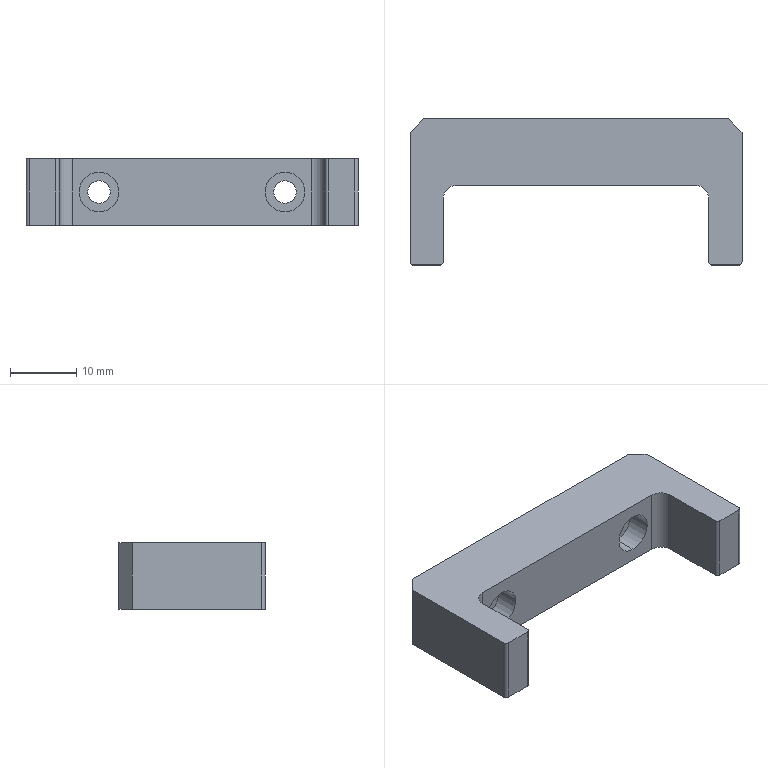Part | SolidWorks | features Fillet 2, Chamfer 1, Extrusion 1, HoleWzd 1 | 1 solid | 28 faces | box 50 x 22 x 10 mm | volume 5859 mm3 | cylinder 14 | plane 14 | commonest cylinder face diameters 1 x4 3.4 x4 6 x4 4 x2
STEP:
#1=CARTESIAN_POINT('',(11.,-6.5,8.));
#2=VERTEX_POINT('',#1);
#3=CARTESIAN_POINT('',(11.,-6.5,2.));
#4=VERTEX_POINT('',#3);
#5=CARTESIAN_POINT('',(11.,-6.5,5.));
#6=DIRECTION('',(0.,-1.,0.));
#7=DIRECTION('',(0.,0.,-1.));
#8=AXIS2_PLACEMENT_3D('',#5,#6,#7);
#9=CIRCLE('',#8,3.);
#10=EDGE_CURVE('',#2,#4,#9,.T.);
#11=ORIENTED_EDGE('',*,*,#10,.F.);
#12=CARTESIAN_POINT('',(11.,-10.,8.));
#13=VERTEX_POINT('',#12);
#14=CARTESIAN_POINT('',(11.,-10.,8.));
#15=DIRECTION('',(0.,-1.,0.));
#16=VECTOR('',#15,1000.);
#17=LINE('',#14,#16);
#18=EDGE_CURVE('',#2,#13,#17,.T.);
#19=ORIENTED_EDGE('',*,*,#18,.T.);
#20=CARTESIAN_POINT('',(11.,-10.,2.));
#21=VERTEX_POINT('',#20);
#22=CARTESIAN_POINT('',(11.,-10.,5.));
#23=DIRECTION('',(0.,-1.,0.));
#24=DIRECTION('',(0.,0.,-1.));
#25=AXIS2_PLACEMENT_3D('',#22,#23,#24);
#26=CIRCLE('',#25,3.);
#27=EDGE_CURVE('',#13,#21,#26,.T.);
#28=ORIENTED_EDGE('',*,*,#27,.T.);
#29=CARTESIAN_POINT('',(11.,-10.,2.));
#30=DIRECTION('',(0.,-1.,0.));
#31=VECTOR('',#30,1000.);
#32=LINE('',#29,#31);
#33=EDGE_CURVE('',#4,#21,#32,.T.);
#34=ORIENTED_EDGE('',*,*,#33,.F.);
#35=EDGE_LOOP('',(#11,#19,#28,#34));
#36=FACE_OUTER_BOUND('',#35,.T.);
#37=CARTESIAN_POINT('',(11.,-10.,5.));
#38=DIRECTION('',(0.,-1.,0.));
#39=DIRECTION('',(0.,0.,-1.));
#40=AXIS2_PLACEMENT_3D('',#37,#38,#39);
#41=CYLINDRICAL_SURFACE('',#40,3.);
#42=ADVANCED_FACE('',(#36),#41,.F.);
#43=CARTESIAN_POINT('',(11.,0.,6.7));
#44=VERTEX_POINT('',#43);
#45=CARTESIAN_POINT('',(11.,0.,3.3));
#46=VERTEX_POINT('',#45);
#47=CARTESIAN_POINT('',(11.,0.,5.));
#48=DIRECTION('',(0.,-1.,0.));
#49=DIRECTION('',(0.,0.,-1.));
#50=AXIS2_PLACEMENT_3D('',#47,#48,#49);
#51=CIRCLE('',#50,1.7);
#52=EDGE_CURVE('',#44,#46,#51,.T.);
#53=ORIENTED_EDGE('',*,*,#52,.F.);
#54=CARTESIAN_POINT('',(11.,-6.5,6.7));
#55=VERTEX_POINT('',#54);
#56=CARTESIAN_POINT('',(11.,-10.,6.7));
#57=DIRECTION('',(0.,-1.,0.));
#58=VECTOR('',#57,1000.);
#59=LINE('',#56,#58);
#60=EDGE_CURVE('',#44,#55,#59,.T.);
#61=ORIENTED_EDGE('',*,*,#60,.T.);
#62=CARTESIAN_POINT('',(11.,-6.5,3.3));
#63=VERTEX_POINT('',#62);
#64=CARTESIAN_POINT('',(11.,-6.5,5.));
#65=DIRECTION('',(0.,-1.,0.));
#66=DIRECTION('',(0.,0.,-1.));
#67=AXIS2_PLACEMENT_3D('',#64,#65,#66);
#68=CIRCLE('',#67,1.7);
#69=EDGE_CURVE('',#55,#63,#68,.T.);
#70=ORIENTED_EDGE('',*,*,#69,.T.);
#71=CARTESIAN_POINT('',(11.,-10.,3.3));
#72=DIRECTION('',(0.,-1.,0.));
#73=VECTOR('',#72,1000.);
#74=LINE('',#71,#73);
#75=EDGE_CURVE('',#46,#63,#74,.T.);
#76=ORIENTED_EDGE('',*,*,#75,.F.);
#77=EDGE_LOOP('',(#53,#61,#70,#76));
#78=FACE_OUTER_BOUND('',#77,.T.);
#79=CARTESIAN_POINT('',(11.,-10.,5.));
#80=DIRECTION('',(0.,-1.,0.));
#81=DIRECTION('',(0.,0.,-1.));
#82=AXIS2_PLACEMENT_3D('',#79,#80,#81);
#83=CYLINDRICAL_SURFACE('',#82,1.7);
#84=ADVANCED_FACE('',(#78),#83,.F.);
#85=CARTESIAN_POINT('',(39.,-6.5,8.));
#86=VERTEX_POINT('',#85);
#87=CARTESIAN_POINT('',(39.,-6.5,2.));
#88=VERTEX_POINT('',#87);
#89=CARTESIAN_POINT('',(39.,-6.5,5.));
#90=DIRECTION('',(0.,-1.,0.));
#91=DIRECTION('',(0.,0.,-1.));
#92=AXIS2_PLACEMENT_3D('',#89,#90,#91);
#93=CIRCLE('',#92,3.);
#94=EDGE_CURVE('',#86,#88,#93,.T.);
#95=ORIENTED_EDGE('',*,*,#94,.F.);
#96=CARTESIAN_POINT('',(39.,-10.,8.));
#97=VERTEX_POINT('',#96);
#98=CARTESIAN_POINT('',(39.,-10.,8.));
#99=DIRECTION('',(0.,-1.,0.));
#100=VECTOR('',#99,1000.);
#101=LINE('',#98,#100);
#102=EDGE_CURVE('',#86,#97,#101,.T.);
#103=ORIENTED_EDGE('',*,*,#102,.T.);
#104=CARTESIAN_POINT('',(39.,-10.,2.));
#105=VERTEX_POINT('',#104);
#106=CARTESIAN_POINT('',(39.,-10.,5.));
#107=DIRECTION('',(0.,-1.,0.));
#108=DIRECTION('',(0.,0.,-1.));
#109=AXIS2_PLACEMENT_3D('',#106,#107,#108);
#110=CIRCLE('',#109,3.);
#111=EDGE_CURVE('',#97,#105,#110,.T.);
#112=ORIENTED_EDGE('',*,*,#111,.T.);
#113=CARTESIAN_POINT('',(39.,-10.,2.));
#114=DIRECTION('',(0.,-1.,0.));
#115=VECTOR('',#114,1000.);
#116=LINE('',#113,#115);
#117=EDGE_CURVE('',#88,#105,#116,.T.);
#118=ORIENTED_EDGE('',*,*,#117,.F.);
#119=EDGE_LOOP('',(#95,#103,#112,#118));
#120=FACE_OUTER_BOUND('',#119,.T.);
#121=CARTESIAN_POINT('',(39.,-10.,5.));
#122=DIRECTION('',(0.,-1.,0.));
#123=DIRECTION('',(0.,0.,-1.));
#124=AXIS2_PLACEMENT_3D('',#121,#122,#123);
#125=CYLINDRICAL_SURFACE('',#124,3.);
#126=ADVANCED_FACE('',(#120),#125,.F.);
#127=CARTESIAN_POINT('',(39.,0.,6.7));
#128=VERTEX_POINT('',#127);
#129=CARTESIAN_POINT('',(39.,0.,3.3));
#130=VERTEX_POINT('',#129);
#131=CARTESIAN_POINT('',(39.,0.,5.));
#132=DIRECTION('',(0.,-1.,0.));
#133=DIRECTION('',(0.,0.,-1.));
#134=AXIS2_PLACEMENT_3D('',#131,#132,#133);
#135=CIRCLE('',#134,1.7);
#136=EDGE_CURVE('',#128,#130,#135,.T.);
#137=ORIENTED_EDGE('',*,*,#136,.F.);
#138=CARTESIAN_POINT('',(39.,-6.5,6.7));
#139=VERTEX_POINT('',#138);
#140=CARTESIAN_POINT('',(39.,-10.,6.7));
#141=DIRECTION('',(0.,-1.,0.));
#142=VECTOR('',#141,1000.);
#143=LINE('',#140,#142);
#144=EDGE_CURVE('',#128,#139,#143,.T.);
#145=ORIENTED_EDGE('',*,*,#144,.T.);
#146=CARTESIAN_POINT('',(39.,-6.5,3.3));
#147=VERTEX_POINT('',#146);
#148=CARTESIAN_POINT('',(39.,-6.5,5.));
#149=DIRECTION('',(0.,-1.,0.));
#150=DIRECTION('',(0.,0.,-1.));
#151=AXIS2_PLACEMENT_3D('',#148,#149,#150);
#152=CIRCLE('',#151,1.7);
#153=EDGE_CURVE('',#139,#147,#152,.T.);
#154=ORIENTED_EDGE('',*,*,#153,.T.);
#155=CARTESIAN_POINT('',(39.,-10.,3.3));
#156=DIRECTION('',(0.,-1.,0.));
#157=VECTOR('',#156,1000.);
#158=LINE('',#155,#157);
#159=EDGE_CURVE('',#130,#147,#158,.T.);
#160=ORIENTED_EDGE('',*,*,#159,.F.);
#161=EDGE_LOOP('',(#137,#145,#154,#160));
#162=FACE_OUTER_BOUND('',#161,.T.);
#163=CARTESIAN_POINT('',(39.,-10.,5.));
#164=DIRECTION('',(0.,-1.,0.));
#165=DIRECTION('',(0.,0.,-1.));
#166=AXIS2_PLACEMENT_3D('',#163,#164,#165);
#167=CYLINDRICAL_SURFACE('',#166,1.7);
#168=ADVANCED_FACE('',(#162),#167,.F.);
#169=CARTESIAN_POINT('',(0.,-2.,10.));
#170=VERTEX_POINT('',#169);
#171=CARTESIAN_POINT('',(0.,-21.5,10.));
#172=VERTEX_POINT('',#171);
#173=CARTESIAN_POINT('',(0.,0.,10.));
#174=DIRECTION('',(0.,-1.,0.));
#175=VECTOR('',#174,1000.);
#176=LINE('',#173,#175);
#177=EDGE_CURVE('',#170,#172,#176,.T.);
#178=ORIENTED_EDGE('',*,*,#177,.F.);
#179=CARTESIAN_POINT('',(0.,-2.,0.));
#180=VERTEX_POINT('',#179);
#181=CARTESIAN_POINT('',(0.,-2.,10.));
#182=DIRECTION('',(0.,0.,-1.));
#183=VECTOR('',#182,1000.);
#184=LINE('',#181,#183);
#185=EDGE_CURVE('',#170,#180,#184,.T.);
#186=ORIENTED_EDGE('',*,*,#185,.T.);
#187=CARTESIAN_POINT('',(0.,-21.5,0.));
#188=VERTEX_POINT('',#187);
#189=CARTESIAN_POINT('',(0.,0.,0.));
#190=DIRECTION('',(0.,-1.,0.));
#191=VECTOR('',#190,1000.);
#192=LINE('',#189,#191);
#193=EDGE_CURVE('',#180,#188,#192,.T.);
#194=ORIENTED_EDGE('',*,*,#193,.T.);
#195=CARTESIAN_POINT('',(0.,-21.5,10.));
#196=DIRECTION('',(0.,0.,1.));
#197=VECTOR('',#196,1000.);
#198=LINE('',#195,#197);
#199=EDGE_CURVE('',#188,#172,#198,.T.);
#200=ORIENTED_EDGE('',*,*,#199,.T.);
#201=EDGE_LOOP('',(#178,#186,#194,#200));
#202=FACE_OUTER_BOUND('',#201,.T.);
#203=CARTESIAN_POINT('',(0.,0.,10.));
#204=DIRECTION('',(1.,0.,0.));
#205=DIRECTION('',(0.,1.,0.));
#206=AXIS2_PLACEMENT_3D('',#203,#204,#205);
#207=PLANE('',#206);
#208=ADVANCED_FACE('',(#202),#207,.F.);
#209=CARTESIAN_POINT('',(0.5,-22.,0.));
#210=VERTEX_POINT('',#209);
#211=CARTESIAN_POINT('',(4.5,-22.,0.));
#212=VERTEX_POINT('',#211);
#213=CARTESIAN_POINT('',(0.,-22.,0.));
#214=DIRECTION('',(1.,0.,0.));
#215=VECTOR('',#214,1000.);
#216=LINE('',#213,#215);
#217=EDGE_CURVE('',#210,#212,#216,.T.);
#218=ORIENTED_EDGE('',*,*,#217,.T.);
#219=CARTESIAN_POINT('',(4.5,-22.,10.));
#220=VERTEX_POINT('',#219);
#221=CARTESIAN_POINT('',(4.5,-22.,10.));
#222=DIRECTION('',(0.,0.,1.));
#223=VECTOR('',#222,1000.);
#224=LINE('',#221,#223);
#225=EDGE_CURVE('',#212,#220,#224,.T.);
#226=ORIENTED_EDGE('',*,*,#225,.T.);
#227=CARTESIAN_POINT('',(0.5,-22.,10.));
#228=VERTEX_POINT('',#227);
#229=CARTESIAN_POINT('',(0.,-22.,10.));
#230=DIRECTION('',(1.,0.,0.));
#231=VECTOR('',#230,1000.);
#232=LINE('',#229,#231);
#233=EDGE_CURVE('',#228,#220,#232,.T.);
#234=ORIENTED_EDGE('',*,*,#233,.F.);
#235=CARTESIAN_POINT('',(0.5,-22.,10.));
#236=DIRECTION('',(0.,0.,-1.));
#237=VECTOR('',#236,1000.);
#238=LINE('',#235,#237);
#239=EDGE_CURVE('',#228,#210,#238,.T.);
#240=ORIENTED_EDGE('',*,*,#239,.T.);
#241=EDGE_LOOP('',(#218,#226,#234,#240));
#242=FACE_OUTER_BOUND('',#241,.T.);
#243=CARTESIAN_POINT('',(0.,-22.,10.));
#244=DIRECTION('',(0.,1.,0.));
#245=DIRECTION('',(0.,0.,1.));
#246=AXIS2_PLACEMENT_3D('',#243,#244,#245);
#247=PLANE('',#246);
#248=ADVANCED_FACE('',(#242),#247,.F.);
#249=CARTESIAN_POINT('',(5.,-21.5,10.));
#250=VERTEX_POINT('',#249);
#251=CARTESIAN_POINT('',(5.,-12.,10.));
#252=VERTEX_POINT('',#251);
#253=CARTESIAN_POINT('',(5.,-22.,10.));
#254=DIRECTION('',(0.,1.,0.));
#255=VECTOR('',#254,1000.);
#256=LINE('',#253,#255);
#257=EDGE_CURVE('',#250,#252,#256,.T.);
#258=ORIENTED_EDGE('',*,*,#257,.F.);
#259=CARTESIAN_POINT('',(5.,-21.5,0.));
#260=VERTEX_POINT('',#259);
#261=CARTESIAN_POINT('',(5.,-21.5,10.));
#262=DIRECTION('',(0.,0.,-1.));
#263=VECTOR('',#262,1000.);
#264=LINE('',#261,#263);
#265=EDGE_CURVE('',#250,#260,#264,.T.);
#266=ORIENTED_EDGE('',*,*,#265,.T.);
#267=CARTESIAN_POINT('',(5.,-12.,0.));
#268=VERTEX_POINT('',#267);
#269=CARTESIAN_POINT('',(5.,-22.,0.));
#270=DIRECTION('',(0.,1.,0.));
#271=VECTOR('',#270,1000.);
#272=LINE('',#269,#271);
#273=EDGE_CURVE('',#260,#268,#272,.T.);
#274=ORIENTED_EDGE('',*,*,#273,.T.);
#275=CARTESIAN_POINT('',(5.,-12.,10.));
#276=DIRECTION('',(0.,0.,1.));
#277=VECTOR('',#276,1000.);
#278=LINE('',#275,#277);
#279=EDGE_CURVE('',#268,#252,#278,.T.);
#280=ORIENTED_EDGE('',*,*,#279,.T.);
#281=EDGE_LOOP('',(#258,#266,#274,#280));
#282=FACE_OUTER_BOUND('',#281,.T.);
#283=CARTESIAN_POINT('',(5.,-22.,10.));
#284=DIRECTION('',(-1.,0.,0.));
#285=DIRECTION('',(0.,0.,1.));
#286=AXIS2_PLACEMENT_3D('',#283,#284,#285);
#287=PLANE('',#286);
#288=ADVANCED_FACE('',(#282),#287,.F.);
#289=CARTESIAN_POINT('',(11.,-10.,5.));
#290=DIRECTION('',(0.,-1.,0.));
#291=DIRECTION('',(0.,0.,-1.));
#292=AXIS2_PLACEMENT_3D('',#289,#290,#291);
#293=CIRCLE('',#292,3.);
#294=EDGE_CURVE('',#21,#13,#293,.T.);
#295=ORIENTED_EDGE('',*,*,#294,.F.);
#296=ORIENTED_EDGE('',*,*,#27,.F.);
#297=EDGE_LOOP('',(#295,#296));
#298=FACE_BOUND('',#297,.T.);
#299=CARTESIAN_POINT('',(39.,-10.,5.));
#300=DIRECTION('',(0.,-1.,0.));
#301=DIRECTION('',(0.,0.,-1.));
#302=AXIS2_PLACEMENT_3D('',#299,#300,#301);
#303=CIRCLE('',#302,3.);
#304=EDGE_CURVE('',#105,#97,#303,.T.);
#305=ORIENTED_EDGE('',*,*,#304,.F.);
#306=ORIENTED_EDGE('',*,*,#111,.F.);
#307=EDGE_LOOP('',(#305,#306));
#308=FACE_BOUND('',#307,.T.);
#309=CARTESIAN_POINT('',(7.,-10.,0.));
#310=VERTEX_POINT('',#309);
#311=CARTESIAN_POINT('',(43.,-10.,0.));
#312=VERTEX_POINT('',#311);
#313=CARTESIAN_POINT('',(5.,-10.,0.));
#314=DIRECTION('',(1.,0.,0.));
#315=VECTOR('',#314,1000.);
#316=LINE('',#313,#315);
#317=EDGE_CURVE('',#310,#312,#316,.T.);
#318=ORIENTED_EDGE('',*,*,#317,.T.);
#319=CARTESIAN_POINT('',(43.,-10.,10.));
#320=VERTEX_POINT('',#319);
#321=CARTESIAN_POINT('',(43.,-10.,10.));
#322=DIRECTION('',(0.,0.,1.));
#323=VECTOR('',#322,1000.);
#324=LINE('',#321,#323);
#325=EDGE_CURVE('',#312,#320,#324,.T.);
#326=ORIENTED_EDGE('',*,*,#325,.T.);
#327=CARTESIAN_POINT('',(7.,-10.,10.));
#328=VERTEX_POINT('',#327);
#329=CARTESIAN_POINT('',(5.,-10.,10.));
#330=DIRECTION('',(1.,0.,0.));
#331=VECTOR('',#330,1000.);
#332=LINE('',#329,#331);
#333=EDGE_CURVE('',#328,#320,#332,.T.);
#334=ORIENTED_EDGE('',*,*,#333,.F.);
#335=CARTESIAN_POINT('',(7.,-10.,0.));
#336=DIRECTION('',(0.,0.,-1.));
#337=VECTOR('',#336,1000.);
#338=LINE('',#335,#337);
#339=EDGE_CURVE('',#328,#310,#338,.T.);
#340=ORIENTED_EDGE('',*,*,#339,.T.);
#341=EDGE_LOOP('',(#318,#326,#334,#340));
#342=FACE_OUTER_BOUND('',#341,.T.);
#343=CARTESIAN_POINT('',(5.,-10.,10.));
#344=DIRECTION('',(0.,1.,0.));
#345=DIRECTION('',(0.,0.,1.));
#346=AXIS2_PLACEMENT_3D('',#343,#344,#345);
#347=PLANE('',#346);
#348=ADVANCED_FACE('',(#298,#308,#342),#347,.F.);
#349=CARTESIAN_POINT('',(45.,-12.,0.));
#350=VERTEX_POINT('',#349);
#351=CARTESIAN_POINT('',(45.,-21.5,0.));
#352=VERTEX_POINT('',#351);
#353=CARTESIAN_POINT('',(45.,-22.,0.));
#354=DIRECTION('',(0.,-1.,0.));
#355=VECTOR('',#354,1000.);
#356=LINE('',#353,#355);
#357=EDGE_CURVE('',#350,#352,#356,.T.);
#358=ORIENTED_EDGE('',*,*,#357,.T.);
#359=CARTESIAN_POINT('',(45.,-21.5,10.));
#360=VERTEX_POINT('',#359);
#361=CARTESIAN_POINT('',(45.,-21.5,10.));
#362=DIRECTION('',(0.,0.,1.));
#363=VECTOR('',#362,1000.);
#364=LINE('',#361,#363);
#365=EDGE_CURVE('',#352,#360,#364,.T.);
#366=ORIENTED_EDGE('',*,*,#365,.T.);
#367=CARTESIAN_POINT('',(45.,-12.,10.));
#368=VERTEX_POINT('',#367);
#369=CARTESIAN_POINT('',(45.,-22.,10.));
#370=DIRECTION('',(0.,-1.,0.));
#371=VECTOR('',#370,1000.);
#372=LINE('',#369,#371);
#373=EDGE_CURVE('',#368,#360,#372,.T.);
#374=ORIENTED_EDGE('',*,*,#373,.F.);
#375=CARTESIAN_POINT('',(45.,-12.,0.));
#376=DIRECTION('',(0.,0.,-1.));
#377=VECTOR('',#376,1000.);
#378=LINE('',#375,#377);
#379=EDGE_CURVE('',#368,#350,#378,.T.);
#380=ORIENTED_EDGE('',*,*,#379,.T.);
#381=EDGE_LOOP('',(#358,#366,#374,#380));
#382=FACE_OUTER_BOUND('',#381,.T.);
#383=CARTESIAN_POINT('',(45.,-22.,10.));
#384=DIRECTION('',(1.,0.,0.));
#385=DIRECTION('',(0.,0.,-1.));
#386=AXIS2_PLACEMENT_3D('',#383,#384,#385);
#387=PLANE('',#386);
#388=ADVANCED_FACE('',(#382),#387,.F.);
#389=CARTESIAN_POINT('',(45.5,-22.,0.));
#390=VERTEX_POINT('',#389);
#391=CARTESIAN_POINT('',(49.5,-22.,0.));
#392=VERTEX_POINT('',#391);
#393=CARTESIAN_POINT('',(45.,-22.,0.));
#394=DIRECTION('',(1.,0.,0.));
#395=VECTOR('',#394,1000.);
#396=LINE('',#393,#395);
#397=EDGE_CURVE('',#390,#392,#396,.T.);
#398=ORIENTED_EDGE('',*,*,#397,.T.);
#399=CARTESIAN_POINT('',(49.5,-22.,10.));
#400=VERTEX_POINT('',#399);
#401=CARTESIAN_POINT('',(49.5,-22.,10.));
#402=DIRECTION('',(0.,0.,1.));
#403=VECTOR('',#402,1000.);
#404=LINE('',#401,#403);
#405=EDGE_CURVE('',#392,#400,#404,.T.);
#406=ORIENTED_EDGE('',*,*,#405,.T.);
#407=CARTESIAN_POINT('',(45.5,-22.,10.));
#408=VERTEX_POINT('',#407);
#409=CARTESIAN_POINT('',(45.,-22.,10.));
#410=DIRECTION('',(1.,0.,0.));
#411=VECTOR('',#410,1000.);
#412=LINE('',#409,#411);
#413=EDGE_CURVE('',#408,#400,#412,.T.);
#414=ORIENTED_EDGE('',*,*,#413,.F.);
#415=CARTESIAN_POINT('',(45.5,-22.,10.));
#416=DIRECTION('',(0.,0.,-1.));
#417=VECTOR('',#416,1000.);
#418=LINE('',#415,#417);
#419=EDGE_CURVE('',#408,#390,#418,.T.);
#420=ORIENTED_EDGE('',*,*,#419,.T.);
#421=EDGE_LOOP('',(#398,#406,#414,#420));
#422=FACE_OUTER_BOUND('',#421,.T.);
#423=CARTESIAN_POINT('',(45.,-22.,10.));
#424=DIRECTION('',(0.,1.,0.));
#425=DIRECTION('',(0.,0.,1.));
#426=AXIS2_PLACEMENT_3D('',#423,#424,#425);
#427=PLANE('',#426);
#428=ADVANCED_FACE('',(#422),#427,.F.);
#429=CARTESIAN_POINT('',(50.,-21.5,0.));
#430=VERTEX_POINT('',#429);
#431=CARTESIAN_POINT('',(50.,-2.,0.));
#432=VERTEX_POINT('',#431);
#433=CARTESIAN_POINT('',(50.,0.,0.));
#434=DIRECTION('',(0.,1.,0.));
#435=VECTOR('',#434,1000.);
#436=LINE('',#433,#435);
#437=EDGE_CURVE('',#430,#432,#436,.T.);
#438=ORIENTED_EDGE('',*,*,#437,.T.);
#439=CARTESIAN_POINT('',(50.,-2.,10.));
#440=VERTEX_POINT('',#439);
#441=CARTESIAN_POINT('',(50.,-2.,10.));
#442=DIRECTION('',(0.,0.,1.));
#443=VECTOR('',#442,1000.);
#444=LINE('',#441,#443);
#445=EDGE_CURVE('',#432,#440,#444,.T.);
#446=ORIENTED_EDGE('',*,*,#445,.T.);
#447=CARTESIAN_POINT('',(50.,-21.5,10.));
#448=VERTEX_POINT('',#447);
#449=CARTESIAN_POINT('',(50.,0.,10.));
#450=DIRECTION('',(0.,1.,0.));
#451=VECTOR('',#450,1000.);
#452=LINE('',#449,#451);
#453=EDGE_CURVE('',#448,#440,#452,.T.);
#454=ORIENTED_EDGE('',*,*,#453,.F.);
#455=CARTESIAN_POINT('',(50.,-21.5,10.));
#456=DIRECTION('',(0.,0.,-1.));
#457=VECTOR('',#456,1000.);
#458=LINE('',#455,#457);
#459=EDGE_CURVE('',#448,#430,#458,.T.);
#460=ORIENTED_EDGE('',*,*,#459,.T.);
#461=EDGE_LOOP('',(#438,#446,#454,#460));
#462=FACE_OUTER_BOUND('',#461,.T.);
#463=CARTESIAN_POINT('',(50.,0.,10.));
#464=DIRECTION('',(-1.,0.,0.));
#465=DIRECTION('',(0.,0.,1.));
#466=AXIS2_PLACEMENT_3D('',#463,#464,#465);
#467=PLANE('',#466);
#468=ADVANCED_FACE('',(#462),#467,.F.);
#469=CARTESIAN_POINT('',(11.,0.,5.));
#470=DIRECTION('',(0.,-1.,0.));
#471=DIRECTION('',(0.,0.,-1.));
#472=AXIS2_PLACEMENT_3D('',#469,#470,#471);
#473=CIRCLE('',#472,1.7);
#474=EDGE_CURVE('',#46,#44,#473,.T.);
#475=ORIENTED_EDGE('',*,*,#474,.T.);
#476=ORIENTED_EDGE('',*,*,#52,.T.);
#477=EDGE_LOOP('',(#475,#476));
#478=FACE_BOUND('',#477,.T.);
#479=CARTESIAN_POINT('',(39.,0.,5.));
#480=DIRECTION('',(0.,-1.,0.));
#481=DIRECTION('',(0.,0.,-1.));
#482=AXIS2_PLACEMENT_3D('',#479,#480,#481);
#483=CIRCLE('',#482,1.7);
#484=EDGE_CURVE('',#130,#128,#483,.T.);
#485=ORIENTED_EDGE('',*,*,#484,.T.);
#486=ORIENTED_EDGE('',*,*,#136,.T.);
#487=EDGE_LOOP('',(#485,#486));
#488=FACE_BOUND('',#487,.T.);
#489=CARTESIAN_POINT('',(48.,0.,10.));
#490=VERTEX_POINT('',#489);
#491=CARTESIAN_POINT('',(2.,0.,10.));
#492=VERTEX_POINT('',#491);
#493=CARTESIAN_POINT('',(0.,0.,10.));
#494=DIRECTION('',(-1.,0.,0.));
#495=VECTOR('',#494,1000.);
#496=LINE('',#493,#495);
#497=EDGE_CURVE('',#490,#492,#496,.T.);
#498=ORIENTED_EDGE('',*,*,#497,.F.);
#499=CARTESIAN_POINT('',(48.,0.,0.));
#500=VERTEX_POINT('',#499);
#501=CARTESIAN_POINT('',(48.,0.,10.));
#502=DIRECTION('',(0.,0.,-1.));
#503=VECTOR('',#502,1000.);
#504=LINE('',#501,#503);
#505=EDGE_CURVE('',#490,#500,#504,.T.);
#506=ORIENTED_EDGE('',*,*,#505,.T.);
#507=CARTESIAN_POINT('',(2.,0.,0.));
#508=VERTEX_POINT('',#507);
#509=CARTESIAN_POINT('',(0.,0.,0.));
#510=DIRECTION('',(-1.,0.,0.));
#511=VECTOR('',#510,1000.);
#512=LINE('',#509,#511);
#513=EDGE_CURVE('',#500,#508,#512,.T.);
#514=ORIENTED_EDGE('',*,*,#513,.T.);
#515=CARTESIAN_POINT('',(2.,0.,10.));
#516=DIRECTION('',(0.,0.,1.));
#517=VECTOR('',#516,1000.);
#518=LINE('',#515,#517);
#519=EDGE_CURVE('',#508,#492,#518,.T.);
#520=ORIENTED_EDGE('',*,*,#519,.T.);
#521=EDGE_LOOP('',(#498,#506,#514,#520));
#522=FACE_OUTER_BOUND('',#521,.T.);
#523=CARTESIAN_POINT('',(0.,0.,10.));
#524=DIRECTION('',(0.,-1.,0.));
#525=DIRECTION('',(0.,0.,-1.));
#526=AXIS2_PLACEMENT_3D('',#523,#524,#525);
#527=PLANE('',#526);
#528=ADVANCED_FACE('',(#478,#488,#522),#527,.F.);
#529=ORIENTED_EDGE('',*,*,#453,.T.);
#530=CARTESIAN_POINT('',(35.,13.,10.));
#531=DIRECTION('',(-0.7071,0.7071,0.));
#532=VECTOR('',#531,1000.);
#533=LINE('',#530,#532);
#534=EDGE_CURVE('',#440,#490,#533,.T.);
#535=ORIENTED_EDGE('',*,*,#534,.T.);
#536=ORIENTED_EDGE('',*,*,#497,.T.);
#537=CARTESIAN_POINT('',(-10.,-12.,10.));
#538=DIRECTION('',(-0.7071,-0.7071,0.));
#539=VECTOR('',#538,1000.);
#540=LINE('',#537,#539);
#541=EDGE_CURVE('',#492,#170,#540,.T.);
#542=ORIENTED_EDGE('',*,*,#541,.T.);
#543=ORIENTED_EDGE('',*,*,#177,.T.);
#544=CARTESIAN_POINT('',(0.5,-21.5,10.));
#545=DIRECTION('',(0.,0.,1.));
#546=DIRECTION('',(1.,0.,0.));
#547=AXIS2_PLACEMENT_3D('',#544,#545,#546);
#548=CIRCLE('',#547,0.5);
#549=EDGE_CURVE('',#172,#228,#548,.T.);
#550=ORIENTED_EDGE('',*,*,#549,.T.);
#551=ORIENTED_EDGE('',*,*,#233,.T.);
#552=CARTESIAN_POINT('',(4.5,-21.5,10.));
#553=DIRECTION('',(0.,0.,1.));
#554=DIRECTION('',(1.,0.,0.));
#555=AXIS2_PLACEMENT_3D('',#552,#553,#554);
#556=CIRCLE('',#555,0.5);
#557=EDGE_CURVE('',#220,#250,#556,.T.);
#558=ORIENTED_EDGE('',*,*,#557,.T.);
#559=ORIENTED_EDGE('',*,*,#257,.T.);
#560=CARTESIAN_POINT('',(7.,-12.,10.));
#561=DIRECTION('',(0.,0.,-1.));
#562=DIRECTION('',(1.,0.,0.));
#563=AXIS2_PLACEMENT_3D('',#560,#561,#562);
#564=CIRCLE('',#563,2.);
#565=EDGE_CURVE('',#252,#328,#564,.T.);
#566=ORIENTED_EDGE('',*,*,#565,.T.);
#567=ORIENTED_EDGE('',*,*,#333,.T.);
#568=CARTESIAN_POINT('',(43.,-12.,10.));
#569=DIRECTION('',(0.,0.,-1.));
#570=DIRECTION('',(1.,0.,0.));
#571=AXIS2_PLACEMENT_3D('',#568,#569,#570);
#572=CIRCLE('',#571,2.);
#573=EDGE_CURVE('',#320,#368,#572,.T.);
#574=ORIENTED_EDGE('',*,*,#573,.T.);
#575=ORIENTED_EDGE('',*,*,#373,.T.);
#576=CARTESIAN_POINT('',(45.5,-21.5,10.));
#577=DIRECTION('',(0.,0.,1.));
#578=DIRECTION('',(1.,0.,0.));
#579=AXIS2_PLACEMENT_3D('',#576,#577,#578);
#580=CIRCLE('',#579,0.5);
#581=EDGE_CURVE('',#360,#408,#580,.T.);
#582=ORIENTED_EDGE('',*,*,#581,.T.);
#583=ORIENTED_EDGE('',*,*,#413,.T.);
#584=CARTESIAN_POINT('',(49.5,-21.5,10.));
#585=DIRECTION('',(0.,0.,1.));
#586=DIRECTION('',(1.,0.,0.));
#587=AXIS2_PLACEMENT_3D('',#584,#585,#586);
#588=CIRCLE('',#587,0.5);
#589=EDGE_CURVE('',#400,#448,#588,.T.);
#590=ORIENTED_EDGE('',*,*,#589,.T.);
#591=EDGE_LOOP('',(#529,#535,#536,#542,#543,#550,#551,#558,#559,#566,#567,#574,#575,#582,#583,#590));
#592=FACE_OUTER_BOUND('',#591,.T.);
#593=CARTESIAN_POINT('',(0.,-22.,10.));
#594=DIRECTION('',(0.,0.,1.));
#595=DIRECTION('',(1.,0.,0.));
#596=AXIS2_PLACEMENT_3D('',#593,#594,#595);
#597=PLANE('',#596);
#598=ADVANCED_FACE('',(#592),#597,.T.);
#599=ORIENTED_EDGE('',*,*,#513,.F.);
#600=CARTESIAN_POINT('',(48.,0.,0.));
#601=DIRECTION('',(0.7071,-0.7071,0.));
#602=VECTOR('',#601,1000.);
#603=LINE('',#600,#602);
#604=EDGE_CURVE('',#500,#432,#603,.T.);
#605=ORIENTED_EDGE('',*,*,#604,.T.);
#606=ORIENTED_EDGE('',*,*,#437,.F.);
#607=CARTESIAN_POINT('',(49.5,-21.5,0.));
#608=DIRECTION('',(0.,0.,-1.));
#609=DIRECTION('',(1.,0.,0.));
#610=AXIS2_PLACEMENT_3D('',#607,#608,#609);
#611=CIRCLE('',#610,0.5);
#612=EDGE_CURVE('',#430,#392,#611,.T.);
#613=ORIENTED_EDGE('',*,*,#612,.T.);
#614=ORIENTED_EDGE('',*,*,#397,.F.);
#615=CARTESIAN_POINT('',(45.5,-21.5,0.));
#616=DIRECTION('',(0.,0.,-1.));
#617=DIRECTION('',(1.,0.,0.));
#618=AXIS2_PLACEMENT_3D('',#615,#616,#617);
#619=CIRCLE('',#618,0.5);
#620=EDGE_CURVE('',#390,#352,#619,.T.);
#621=ORIENTED_EDGE('',*,*,#620,.T.);
#622=ORIENTED_EDGE('',*,*,#357,.F.);
#623=CARTESIAN_POINT('',(43.,-12.,0.));
#624=DIRECTION('',(0.,0.,1.));
#625=DIRECTION('',(1.,0.,0.));
#626=AXIS2_PLACEMENT_3D('',#623,#624,#625);
#627=CIRCLE('',#626,2.);
#628=EDGE_CURVE('',#350,#312,#627,.T.);
#629=ORIENTED_EDGE('',*,*,#628,.T.);
#630=ORIENTED_EDGE('',*,*,#317,.F.);
#631=CARTESIAN_POINT('',(7.,-12.,0.));
#632=DIRECTION('',(0.,0.,1.));
#633=DIRECTION('',(1.,0.,0.));
#634=AXIS2_PLACEMENT_3D('',#631,#632,#633);
#635=CIRCLE('',#634,2.);
#636=EDGE_CURVE('',#310,#268,#635,.T.);
#637=ORIENTED_EDGE('',*,*,#636,.T.);
#638=ORIENTED_EDGE('',*,*,#273,.F.);
#639=CARTESIAN_POINT('',(4.5,-21.5,0.));
#640=DIRECTION('',(0.,0.,-1.));
#641=DIRECTION('',(1.,0.,0.));
#642=AXIS2_PLACEMENT_3D('',#639,#640,#641);
#643=CIRCLE('',#642,0.5);
#644=EDGE_CURVE('',#260,#212,#643,.T.);
#645=ORIENTED_EDGE('',*,*,#644,.T.);
#646=ORIENTED_EDGE('',*,*,#217,.F.);
#647=CARTESIAN_POINT('',(0.5,-21.5,0.));
#648=DIRECTION('',(0.,0.,-1.));
#649=DIRECTION('',(1.,0.,0.));
#650=AXIS2_PLACEMENT_3D('',#647,#648,#649);
#651=CIRCLE('',#650,0.5);
#652=EDGE_CURVE('',#210,#188,#651,.T.);
#653=ORIENTED_EDGE('',*,*,#652,.T.);
#654=ORIENTED_EDGE('',*,*,#193,.F.);
#655=CARTESIAN_POINT('',(0.,-2.,0.));
#656=DIRECTION('',(0.7071,0.7071,0.));
#657=VECTOR('',#656,1000.);
#658=LINE('',#655,#657);
#659=EDGE_CURVE('',#180,#508,#658,.T.);
#660=ORIENTED_EDGE('',*,*,#659,.T.);
#661=EDGE_LOOP('',(#599,#605,#606,#613,#614,#621,#622,#629,#630,#637,#638,#645,#646,#653,#654,#660));
#662=FACE_OUTER_BOUND('',#661,.T.);
#663=CARTESIAN_POINT('',(0.,-22.,0.));
#664=DIRECTION('',(0.,0.,1.));
#665=DIRECTION('',(1.,0.,0.));
#666=AXIS2_PLACEMENT_3D('',#663,#664,#665);
#667=PLANE('',#666);
#668=ADVANCED_FACE('',(#662),#667,.F.);
#669=ORIENTED_EDGE('',*,*,#144,.F.);
#670=ORIENTED_EDGE('',*,*,#484,.F.);
#671=ORIENTED_EDGE('',*,*,#159,.T.);
#672=CARTESIAN_POINT('',(39.,-6.5,5.));
#673=DIRECTION('',(0.,-1.,0.));
#674=DIRECTION('',(0.,0.,-1.));
#675=AXIS2_PLACEMENT_3D('',#672,#673,#674);
#676=CIRCLE('',#675,1.7);
#677=EDGE_CURVE('',#147,#139,#676,.T.);
#678=ORIENTED_EDGE('',*,*,#677,.T.);
#679=EDGE_LOOP('',(#669,#670,#671,#678));
#680=FACE_OUTER_BOUND('',#679,.T.);
#681=CARTESIAN_POINT('',(39.,-10.,5.));
#682=DIRECTION('',(0.,-1.,0.));
#683=DIRECTION('',(0.,0.,-1.));
#684=AXIS2_PLACEMENT_3D('',#681,#682,#683);
#685=CYLINDRICAL_SURFACE('',#684,1.7);
#686=ADVANCED_FACE('',(#680),#685,.F.);
#687=ORIENTED_EDGE('',*,*,#677,.F.);
#688=ORIENTED_EDGE('',*,*,#153,.F.);
#689=EDGE_LOOP('',(#687,#688));
#690=FACE_BOUND('',#689,.T.);
#691=CARTESIAN_POINT('',(39.,-6.5,5.));
#692=DIRECTION('',(0.,-1.,0.));
#693=DIRECTION('',(0.,0.,-1.));
#694=AXIS2_PLACEMENT_3D('',#691,#692,#693);
#695=CIRCLE('',#694,3.);
#696=EDGE_CURVE('',#88,#86,#695,.T.);
#697=ORIENTED_EDGE('',*,*,#696,.T.);
#698=ORIENTED_EDGE('',*,*,#94,.T.);
#699=EDGE_LOOP('',(#697,#698));
#700=FACE_OUTER_BOUND('',#699,.T.);
#701=CARTESIAN_POINT('',(40.7,-6.5,5.));
#702=DIRECTION('',(0.,1.,0.));
#703=DIRECTION('',(0.,0.,1.));
#704=AXIS2_PLACEMENT_3D('',#701,#702,#703);
#705=PLANE('',#704);
#706=ADVANCED_FACE('',(#690,#700),#705,.F.);
#707=ORIENTED_EDGE('',*,*,#102,.F.);
#708=ORIENTED_EDGE('',*,*,#696,.F.);
#709=ORIENTED_EDGE('',*,*,#117,.T.);
#710=ORIENTED_EDGE('',*,*,#304,.T.);
#711=EDGE_LOOP('',(#707,#708,#709,#710));
#712=FACE_OUTER_BOUND('',#711,.T.);
#713=CARTESIAN_POINT('',(39.,-10.,5.));
#714=DIRECTION('',(0.,-1.,0.));
#715=DIRECTION('',(0.,0.,-1.));
#716=AXIS2_PLACEMENT_3D('',#713,#714,#715);
#717=CYLINDRICAL_SURFACE('',#716,3.);
#718=ADVANCED_FACE('',(#712),#717,.F.);
#719=ORIENTED_EDGE('',*,*,#60,.F.);
#720=ORIENTED_EDGE('',*,*,#474,.F.);
#721=ORIENTED_EDGE('',*,*,#75,.T.);
#722=CARTESIAN_POINT('',(11.,-6.5,5.));
#723=DIRECTION('',(0.,-1.,0.));
#724=DIRECTION('',(0.,0.,-1.));
#725=AXIS2_PLACEMENT_3D('',#722,#723,#724);
#726=CIRCLE('',#725,1.7);
#727=EDGE_CURVE('',#63,#55,#726,.T.);
#728=ORIENTED_EDGE('',*,*,#727,.T.);
#729=EDGE_LOOP('',(#719,#720,#721,#728));
#730=FACE_OUTER_BOUND('',#729,.T.);
#731=CARTESIAN_POINT('',(11.,-10.,5.));
#732=DIRECTION('',(0.,-1.,0.));
#733=DIRECTION('',(0.,0.,-1.));
#734=AXIS2_PLACEMENT_3D('',#731,#732,#733);
#735=CYLINDRICAL_SURFACE('',#734,1.7);
#736=ADVANCED_FACE('',(#730),#735,.F.);
#737=ORIENTED_EDGE('',*,*,#727,.F.);
#738=ORIENTED_EDGE('',*,*,#69,.F.);
#739=EDGE_LOOP('',(#737,#738));
#740=FACE_BOUND('',#739,.T.);
#741=CARTESIAN_POINT('',(11.,-6.5,5.));
#742=DIRECTION('',(0.,-1.,0.));
#743=DIRECTION('',(0.,0.,-1.));
#744=AXIS2_PLACEMENT_3D('',#741,#742,#743);
#745=CIRCLE('',#744,3.);
#746=EDGE_CURVE('',#4,#2,#745,.T.);
#747=ORIENTED_EDGE('',*,*,#746,.T.);
#748=ORIENTED_EDGE('',*,*,#10,.T.);
#749=EDGE_LOOP('',(#747,#748));
#750=FACE_OUTER_BOUND('',#749,.T.);
#751=CARTESIAN_POINT('',(12.7,-6.5,5.));
#752=DIRECTION('',(0.,1.,0.));
#753=DIRECTION('',(0.,0.,1.));
#754=AXIS2_PLACEMENT_3D('',#751,#752,#753);
#755=PLANE('',#754);
#756=ADVANCED_FACE('',(#740,#750),#755,.F.);
#757=ORIENTED_EDGE('',*,*,#18,.F.);
#758=ORIENTED_EDGE('',*,*,#746,.F.);
#759=ORIENTED_EDGE('',*,*,#33,.T.);
#760=ORIENTED_EDGE('',*,*,#294,.T.);
#761=EDGE_LOOP('',(#757,#758,#759,#760));
#762=FACE_OUTER_BOUND('',#761,.T.);
#763=CARTESIAN_POINT('',(11.,-10.,5.));
#764=DIRECTION('',(0.,-1.,0.));
#765=DIRECTION('',(0.,0.,-1.));
#766=AXIS2_PLACEMENT_3D('',#763,#764,#765);
#767=CYLINDRICAL_SURFACE('',#766,3.);
#768=ADVANCED_FACE('',(#762),#767,.F.);
#769=ORIENTED_EDGE('',*,*,#573,.F.);
#770=ORIENTED_EDGE('',*,*,#325,.F.);
#771=ORIENTED_EDGE('',*,*,#628,.F.);
#772=ORIENTED_EDGE('',*,*,#379,.F.);
#773=EDGE_LOOP('',(#769,#770,#771,#772));
#774=FACE_OUTER_BOUND('',#773,.T.);
#775=CARTESIAN_POINT('',(43.,-12.,10.));
#776=DIRECTION('',(0.,0.,1.));
#777=DIRECTION('',(1.,0.,0.));
#778=AXIS2_PLACEMENT_3D('',#775,#776,#777);
#779=CYLINDRICAL_SURFACE('',#778,2.);
#780=ADVANCED_FACE('',(#774),#779,.F.);
#781=ORIENTED_EDGE('',*,*,#565,.F.);
#782=ORIENTED_EDGE('',*,*,#279,.F.);
#783=ORIENTED_EDGE('',*,*,#636,.F.);
#784=ORIENTED_EDGE('',*,*,#339,.F.);
#785=EDGE_LOOP('',(#781,#782,#783,#784));
#786=FACE_OUTER_BOUND('',#785,.T.);
#787=CARTESIAN_POINT('',(7.,-12.,10.));
#788=DIRECTION('',(0.,0.,1.));
#789=DIRECTION('',(1.,0.,0.));
#790=AXIS2_PLACEMENT_3D('',#787,#788,#789);
#791=CYLINDRICAL_SURFACE('',#790,2.);
#792=ADVANCED_FACE('',(#786),#791,.F.);
#793=ORIENTED_EDGE('',*,*,#589,.F.);
#794=ORIENTED_EDGE('',*,*,#405,.F.);
#795=ORIENTED_EDGE('',*,*,#612,.F.);
#796=ORIENTED_EDGE('',*,*,#459,.F.);
#797=EDGE_LOOP('',(#793,#794,#795,#796));
#798=FACE_OUTER_BOUND('',#797,.T.);
#799=CARTESIAN_POINT('',(49.5,-21.5,10.));
#800=DIRECTION('',(0.,0.,-1.));
#801=DIRECTION('',(-1.,0.,0.));
#802=AXIS2_PLACEMENT_3D('',#799,#800,#801);
#803=CYLINDRICAL_SURFACE('',#802,0.5);
#804=ADVANCED_FACE('',(#798),#803,.T.);
#805=ORIENTED_EDGE('',*,*,#581,.F.);
#806=ORIENTED_EDGE('',*,*,#365,.F.);
#807=ORIENTED_EDGE('',*,*,#620,.F.);
#808=ORIENTED_EDGE('',*,*,#419,.F.);
#809=EDGE_LOOP('',(#805,#806,#807,#808));
#810=FACE_OUTER_BOUND('',#809,.T.);
#811=CARTESIAN_POINT('',(45.5,-21.5,10.));
#812=DIRECTION('',(0.,0.,-1.));
#813=DIRECTION('',(-1.,0.,0.));
#814=AXIS2_PLACEMENT_3D('',#811,#812,#813);
#815=CYLINDRICAL_SURFACE('',#814,0.5);
#816=ADVANCED_FACE('',(#810),#815,.T.);
#817=ORIENTED_EDGE('',*,*,#557,.F.);
#818=ORIENTED_EDGE('',*,*,#225,.F.);
#819=ORIENTED_EDGE('',*,*,#644,.F.);
#820=ORIENTED_EDGE('',*,*,#265,.F.);
#821=EDGE_LOOP('',(#817,#818,#819,#820));
#822=FACE_OUTER_BOUND('',#821,.T.);
#823=CARTESIAN_POINT('',(4.5,-21.5,10.));
#824=DIRECTION('',(0.,0.,-1.));
#825=DIRECTION('',(-1.,0.,0.));
#826=AXIS2_PLACEMENT_3D('',#823,#824,#825);
#827=CYLINDRICAL_SURFACE('',#826,0.5);
#828=ADVANCED_FACE('',(#822),#827,.T.);
#829=ORIENTED_EDGE('',*,*,#549,.F.);
#830=ORIENTED_EDGE('',*,*,#199,.F.);
#831=ORIENTED_EDGE('',*,*,#652,.F.);
#832=ORIENTED_EDGE('',*,*,#239,.F.);
#833=EDGE_LOOP('',(#829,#830,#831,#832));
#834=FACE_OUTER_BOUND('',#833,.T.);
#835=CARTESIAN_POINT('',(0.5,-21.5,10.));
#836=DIRECTION('',(0.,0.,-1.));
#837=DIRECTION('',(-1.,0.,0.));
#838=AXIS2_PLACEMENT_3D('',#835,#836,#837);
#839=CYLINDRICAL_SURFACE('',#838,0.5);
#840=ADVANCED_FACE('',(#834),#839,.T.);
#841=ORIENTED_EDGE('',*,*,#534,.F.);
#842=ORIENTED_EDGE('',*,*,#445,.F.);
#843=ORIENTED_EDGE('',*,*,#604,.F.);
#844=ORIENTED_EDGE('',*,*,#505,.F.);
#845=EDGE_LOOP('',(#841,#842,#843,#844));
#846=FACE_OUTER_BOUND('',#845,.T.);
#847=CARTESIAN_POINT('',(48.,0.,10.));
#848=DIRECTION('',(-0.7071,-0.7071,0.));
#849=DIRECTION('',(0.7071,-0.7071,0.));
#850=AXIS2_PLACEMENT_3D('',#847,#848,#849);
#851=PLANE('',#850);
#852=ADVANCED_FACE('',(#846),#851,.F.);
#853=ORIENTED_EDGE('',*,*,#541,.F.);
#854=ORIENTED_EDGE('',*,*,#519,.F.);
#855=ORIENTED_EDGE('',*,*,#659,.F.);
#856=ORIENTED_EDGE('',*,*,#185,.F.);
#857=EDGE_LOOP('',(#853,#854,#855,#856));
#858=FACE_OUTER_BOUND('',#857,.T.);
#859=CARTESIAN_POINT('',(0.,-2.,10.));
#860=DIRECTION('',(0.7071,-0.7071,0.));
#861=DIRECTION('',(0.7071,0.7071,0.));
#862=AXIS2_PLACEMENT_3D('',#859,#860,#861);
#863=PLANE('',#862);
#864=ADVANCED_FACE('',(#858),#863,.F.);
#865=CLOSED_SHELL('',(#42,#84,#126,#168,#208,#248,#288,#348,#388,#428,#468,#528,#598,#668,#686,#706,#718,#736,#756,#768,#780,#792,#804,#816,#828,#840,#852,#864));
#866=MANIFOLD_SOLID_BREP('',#865);
#867=CARTESIAN_POINT('',(0.,0.,0.));
#868=DIRECTION('',(0.,0.,1.));
#869=DIRECTION('',(1.,0.,0.));
#870=AXIS2_PLACEMENT_3D('',#867,#868,#869);
#871=(LENGTH_UNIT()NAMED_UNIT(*)SI_UNIT(.MILLI.,.METRE.));
#872=UNCERTAINTY_MEASURE_WITH_UNIT(LENGTH_MEASURE(0.00001),#871,'','');
#873=(NAMED_UNIT(*)PLANE_ANGLE_UNIT()SI_UNIT($,.RADIAN.));
#874=(NAMED_UNIT(*)SI_UNIT($,.STERADIAN.)SOLID_ANGLE_UNIT());
#875=(GEOMETRIC_REPRESENTATION_CONTEXT(3)GLOBAL_UNCERTAINTY_ASSIGNED_CONTEXT((#872))GLOBAL_UNIT_ASSIGNED_CONTEXT((#871,#873,#874))REPRESENTATION_CONTEXT('',''));
#876=ADVANCED_BREP_SHAPE_REPRESENTATION('',(#866,#870),#875);